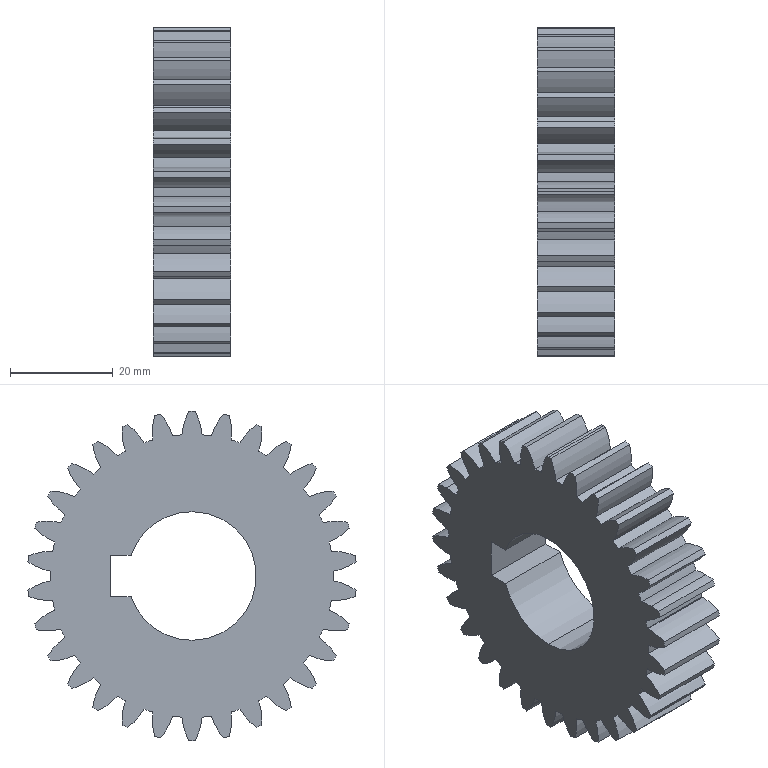Part | SolidWorks | features MBimport 1 | 1 solid | 133 faces | box 15 x 63.764 x 64 mm | volume 33715 mm3 | cylinder 128 | plane 5 | commonest cylinder face diameters 24 x64 64 x31 54.998 x30 25 x3